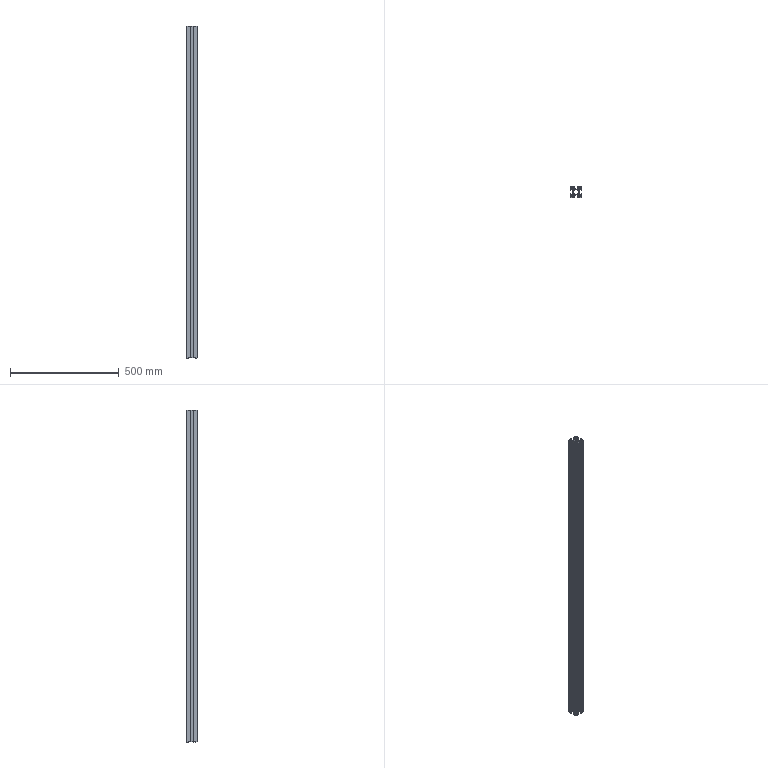Part | STEP file | 46A-00006CC11-1526mm | 1 solid | 142 faces | box 50 x 50 x 1526 mm | volume 896513 mm3 | cylinder 84 | plane 58 | commonest cylinder face diameters 1 x24 4 x24 1.5 x16 3.7 x8 6.7 x8 2 x4